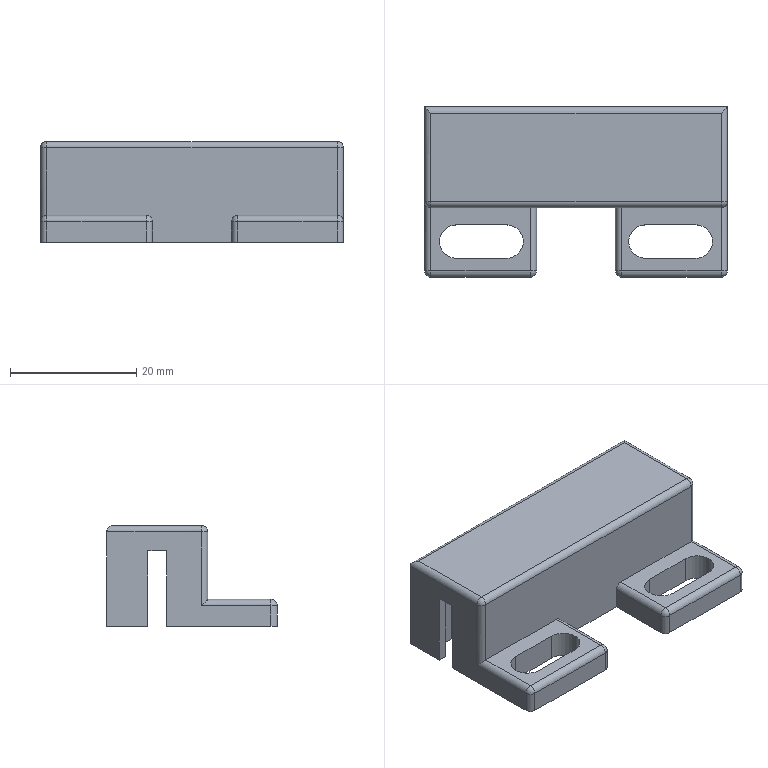Part | NX | features BREP 1 | 1 solid | 96 faces | box 48 x 27 x 16 mm | volume 10049 mm3 | plane 68 | cylinder 22 | sphere 6 | commonest cylinder face diameters 2 x16 5.3 x6